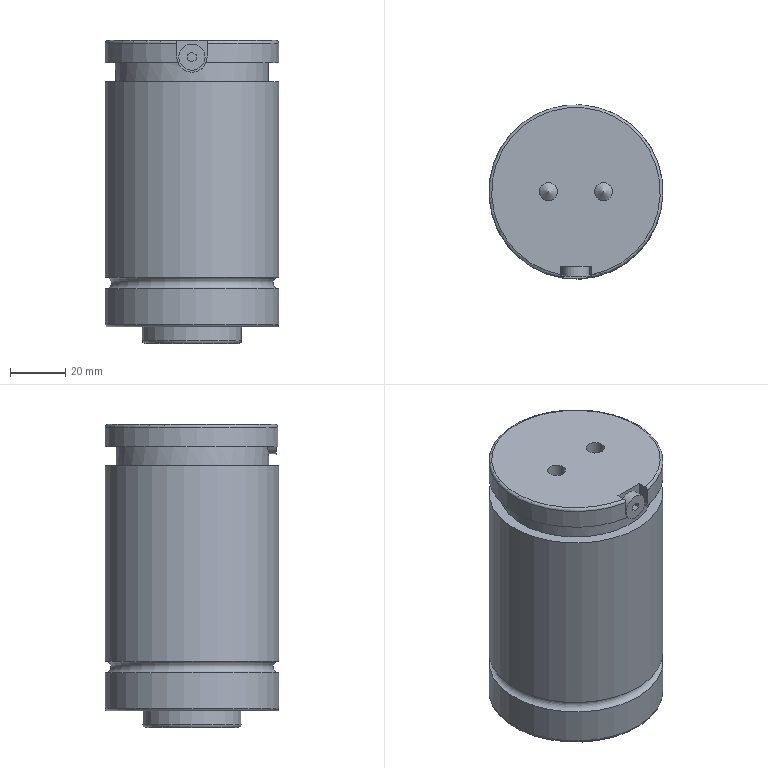Part | NX | features 1 2 | 1 solid | 34 faces | box 63.2 x 63.2 x 110 mm | volume 324925 mm3 | plane 16 | cylinder 10 | torus 4 | cone 4 | commonest cylinder face diameters 63.2 x3 6.6 x2 4.9 x1 9.5 x1 11 x1 36 x1
STEP:
#1=CARTESIAN_POINT('',(-118.4,740.,249.3));
#2=VERTEX_POINT('',#1);
#3=CARTESIAN_POINT('',(-150.,740.,249.3));
#4=DIRECTION('',(0.,0.,-1.));
#5=DIRECTION('',(1.,0.,0.));
#6=AXIS2_PLACEMENT_3D('',#3,#4,#5);
#7=CIRCLE('',#6,31.6);
#8=EDGE_CURVE('',#2,#2,#7,.T.);
#9=ORIENTED_EDGE('',*,*,#8,.T.);
#10=EDGE_LOOP('',(#9));
#11=FACE_BOUND('',#10,.T.);
#12=CARTESIAN_POINT('',(-118.4,740.,245.1));
#13=VERTEX_POINT('',#12);
#14=CARTESIAN_POINT('',(-150.,740.,245.1));
#15=DIRECTION('',(0.,0.,-1.));
#16=DIRECTION('',(1.,0.,0.));
#17=AXIS2_PLACEMENT_3D('',#14,#15,#16);
#18=CIRCLE('',#17,31.6);
#19=EDGE_CURVE('',#13,#13,#18,.T.);
#20=ORIENTED_EDGE('',*,*,#19,.F.);
#21=EDGE_LOOP('',(#20));
#22=FACE_BOUND('',#21,.T.);
#23=CARTESIAN_POINT('',(-150.,740.,247.2));
#24=DIRECTION('',(0.,0.,-1.));
#25=DIRECTION('',(0.,1.,0.));
#26=AXIS2_PLACEMENT_3D('',#23,#24,#25);
#27=TOROIDAL_SURFACE('',#26,31.6,2.1);
#28=ADVANCED_FACE('',(#11,#22),#27,.F.);
#29=CARTESIAN_POINT('',(-118.4,740.,232.2));
#30=VERTEX_POINT('',#29);
#31=CARTESIAN_POINT('',(-150.,740.,232.2));
#32=DIRECTION('',(0.,0.,-1.));
#33=DIRECTION('',(1.,0.,0.));
#34=AXIS2_PLACEMENT_3D('',#31,#32,#33);
#35=CIRCLE('',#34,31.6);
#36=EDGE_CURVE('',#30,#30,#35,.T.);
#37=ORIENTED_EDGE('',*,*,#36,.T.);
#38=EDGE_LOOP('',(#37));
#39=FACE_BOUND('',#38,.T.);
#40=CARTESIAN_POINT('',(-119.4,740.,231.2));
#41=VERTEX_POINT('',#40);
#42=CARTESIAN_POINT('',(-150.,740.,231.2));
#43=DIRECTION('',(0.,0.,-1.));
#44=DIRECTION('',(1.,0.,0.));
#45=AXIS2_PLACEMENT_3D('',#42,#43,#44);
#46=CIRCLE('',#45,30.6);
#47=EDGE_CURVE('',#41,#41,#46,.T.);
#48=ORIENTED_EDGE('',*,*,#47,.F.);
#49=EDGE_LOOP('',(#48));
#50=FACE_BOUND('',#49,.T.);
#51=CARTESIAN_POINT('',(-150.,740.,232.2));
#52=DIRECTION('',(0.,0.,-1.));
#53=DIRECTION('',(0.,1.,0.));
#54=AXIS2_PLACEMENT_3D('',#51,#52,#53);
#55=TOROIDAL_SURFACE('',#54,30.6,1.);
#56=ADVANCED_FACE('',(#39,#50),#55,.T.);
#57=ORIENTED_EDGE('',*,*,#19,.T.);
#58=EDGE_LOOP('',(#57));
#59=FACE_BOUND('',#58,.T.);
#60=ORIENTED_EDGE('',*,*,#36,.F.);
#61=EDGE_LOOP('',(#60));
#62=FACE_BOUND('',#61,.T.);
#63=CARTESIAN_POINT('',(-150.,740.,238.65));
#64=DIRECTION('',(0.,0.,1.));
#65=DIRECTION('',(0.,-1.,0.));
#66=AXIS2_PLACEMENT_3D('',#63,#64,#65);
#67=CYLINDRICAL_SURFACE('',#66,31.6);
#68=ADVANCED_FACE('',(#59,#62),#67,.T.);
#69=CARTESIAN_POINT('',(-118.4,740.,320.2));
#70=VERTEX_POINT('',#69);
#71=CARTESIAN_POINT('',(-150.,740.,320.2));
#72=DIRECTION('',(0.,0.,1.));
#73=DIRECTION('',(1.,0.,0.));
#74=AXIS2_PLACEMENT_3D('',#71,#72,#73);
#75=CIRCLE('',#74,31.6);
#76=EDGE_CURVE('',#70,#70,#75,.F.);
#77=ORIENTED_EDGE('',*,*,#76,.T.);
#78=EDGE_LOOP('',(#77));
#79=FACE_BOUND('',#78,.T.);
#80=ORIENTED_EDGE('',*,*,#8,.F.);
#81=EDGE_LOOP('',(#80));
#82=FACE_BOUND('',#81,.T.);
#83=CARTESIAN_POINT('',(-150.,740.,310.25));
#84=DIRECTION('',(0.,0.,1.));
#85=DIRECTION('',(0.,-1.,0.));
#86=AXIS2_PLACEMENT_3D('',#83,#84,#85);
#87=CYLINDRICAL_SURFACE('',#86,31.6);
#88=ADVANCED_FACE('',(#79,#82),#87,.T.);
#89=CARTESIAN_POINT('',(-122.2,740.,320.2));
#90=VERTEX_POINT('',#89);
#91=CARTESIAN_POINT('',(-150.,740.,320.2));
#92=DIRECTION('',(0.,0.,-1.));
#93=DIRECTION('',(1.,0.,0.));
#94=AXIS2_PLACEMENT_3D('',#91,#92,#93);
#95=CIRCLE('',#94,27.8);
#96=EDGE_CURVE('',#90,#90,#95,.T.);
#97=ORIENTED_EDGE('',*,*,#96,.F.);
#98=EDGE_LOOP('',(#97));
#99=FACE_BOUND('',#98,.T.);
#100=CARTESIAN_POINT('',(-155.123,712.676,327.2));
#101=VERTEX_POINT('',#100);
#102=CARTESIAN_POINT('',(-144.877,712.676,327.2));
#103=VERTEX_POINT('',#102);
#104=CARTESIAN_POINT('',(-150.,740.,327.2));
#105=DIRECTION('',(0.,0.,-1.));
#106=DIRECTION('',(1.,0.,0.));
#107=AXIS2_PLACEMENT_3D('',#104,#105,#106);
#108=CIRCLE('',#107,27.8);
#109=EDGE_CURVE('',#101,#103,#108,.T.);
#110=ORIENTED_EDGE('',*,*,#109,.T.);
#111=CARTESIAN_POINT('',(-144.877,712.676,327.2));
#112=CARTESIAN_POINT('',(-145.28,712.601,326.166));
#113=CARTESIAN_POINT('',(-146.696,712.348,324.391));
#114=CARTESIAN_POINT('',(-149.997,712.126,323.355));
#115=CARTESIAN_POINT('',(-153.301,712.348,324.388));
#116=CARTESIAN_POINT('',(-154.72,712.601,326.166));
#117=CARTESIAN_POINT('',(-155.123,712.676,327.2));
#118=B_SPLINE_CURVE_WITH_KNOTS('',3,(#111,#112,#113,#114,#115,#116,#117),.UNSPECIFIED.,.F.,.F.,(4,1,1,1,4),(0.,0.00329,0.006579,0.009869,0.01316),.UNSPECIFIED.);
#119=EDGE_CURVE('',#103,#101,#118,.T.);
#120=ORIENTED_EDGE('',*,*,#119,.T.);
#121=EDGE_LOOP('',(#110,#120));
#122=FACE_BOUND('',#121,.T.);
#123=CARTESIAN_POINT('',(-150.,740.,323.7));
#124=DIRECTION('',(0.,0.,1.));
#125=DIRECTION('',(0.,-1.,0.));
#126=AXIS2_PLACEMENT_3D('',#123,#124,#125);
#127=CYLINDRICAL_SURFACE('',#126,27.8);
#128=ADVANCED_FACE('',(#99,#122),#127,.T.);
#129=CARTESIAN_POINT('',(-132.,740.,226.2));
#130=VERTEX_POINT('',#129);
#131=CARTESIAN_POINT('',(-150.,740.,226.2));
#132=DIRECTION('',(0.,0.,-1.));
#133=DIRECTION('',(1.,0.,0.));
#134=AXIS2_PLACEMENT_3D('',#131,#132,#133);
#135=CIRCLE('',#134,18.);
#136=EDGE_CURVE('',#130,#130,#135,.T.);
#137=ORIENTED_EDGE('',*,*,#136,.T.);
#138=EDGE_LOOP('',(#137));
#139=FACE_BOUND('',#138,.T.);
#140=CARTESIAN_POINT('',(-133.,740.,225.2));
#141=VERTEX_POINT('',#140);
#142=CARTESIAN_POINT('',(-150.,740.,225.2));
#143=DIRECTION('',(0.,0.,-1.));
#144=DIRECTION('',(1.,0.,0.));
#145=AXIS2_PLACEMENT_3D('',#142,#143,#144);
#146=CIRCLE('',#145,17.);
#147=EDGE_CURVE('',#141,#141,#146,.T.);
#148=ORIENTED_EDGE('',*,*,#147,.F.);
#149=EDGE_LOOP('',(#148));
#150=FACE_BOUND('',#149,.T.);
#151=CARTESIAN_POINT('',(-150.,740.,226.2));
#152=DIRECTION('',(0.,0.,-1.));
#153=DIRECTION('',(0.,1.,0.));
#154=AXIS2_PLACEMENT_3D('',#151,#152,#153);
#155=TOROIDAL_SURFACE('',#154,17.,1.);
#156=ADVANCED_FACE('',(#139,#150),#155,.T.);
#157=CARTESIAN_POINT('',(-132.,740.,231.2));
#158=VERTEX_POINT('',#157);
#159=CARTESIAN_POINT('',(-150.,740.,231.2));
#160=DIRECTION('',(0.,0.,1.));
#161=DIRECTION('',(1.,0.,0.));
#162=AXIS2_PLACEMENT_3D('',#159,#160,#161);
#163=CIRCLE('',#162,18.);
#164=EDGE_CURVE('',#158,#158,#163,.T.);
#165=ORIENTED_EDGE('',*,*,#164,.F.);
#166=EDGE_LOOP('',(#165));
#167=FACE_BOUND('',#166,.T.);
#168=ORIENTED_EDGE('',*,*,#136,.F.);
#169=EDGE_LOOP('',(#168));
#170=FACE_BOUND('',#169,.T.);
#171=CARTESIAN_POINT('',(-150.,740.,230.2));
#172=DIRECTION('',(0.,0.,1.));
#173=DIRECTION('',(0.,-1.,0.));
#174=AXIS2_PLACEMENT_3D('',#171,#172,#173);
#175=CYLINDRICAL_SURFACE('',#174,18.);
#176=ADVANCED_FACE('',(#167,#170),#175,.T.);
#177=CARTESIAN_POINT('',(-143.3,740.,335.2));
#178=VERTEX_POINT('',#177);
#179=CARTESIAN_POINT('',(-140.,740.,335.2));
#180=DIRECTION('',(0.,0.,-1.));
#181=DIRECTION('',(-1.,0.,0.));
#182=AXIS2_PLACEMENT_3D('',#179,#180,#181);
#183=CIRCLE('',#182,3.3);
#184=EDGE_CURVE('',#178,#178,#183,.T.);
#185=ORIENTED_EDGE('',*,*,#184,.F.);
#186=EDGE_LOOP('',(#185));
#187=FACE_BOUND('',#186,.T.);
#188=CARTESIAN_POINT('',(-143.3,740.,324.));
#189=VERTEX_POINT('',#188);
#190=CARTESIAN_POINT('',(-140.,740.,324.));
#191=DIRECTION('',(0.,0.,1.));
#192=DIRECTION('',(-1.,0.,0.));
#193=AXIS2_PLACEMENT_3D('',#190,#191,#192);
#194=CIRCLE('',#193,3.3);
#195=EDGE_CURVE('',#189,#189,#194,.T.);
#196=ORIENTED_EDGE('',*,*,#195,.F.);
#197=EDGE_LOOP('',(#196));
#198=FACE_BOUND('',#197,.T.);
#199=CARTESIAN_POINT('',(-140.,740.,329.6));
#200=DIRECTION('',(0.,0.,-1.));
#201=DIRECTION('',(0.,1.,0.));
#202=AXIS2_PLACEMENT_3D('',#199,#200,#201);
#203=CYLINDRICAL_SURFACE('',#202,3.3);
#204=ADVANCED_FACE('',(#187,#198),#203,.F.);
#205=ORIENTED_EDGE('',*,*,#195,.T.);
#206=EDGE_LOOP('',(#205));
#207=FACE_BOUND('',#206,.T.);
#208=CARTESIAN_POINT('',(-140.,740.,326.7));
#209=VERTEX_POINT('',#208);
#210=VERTEX_LOOP('',#209);
#211=FACE_BOUND('',#210,.T.);
#212=CARTESIAN_POINT('',(-140.,740.,325.35));
#213=DIRECTION('',(0.,0.,-1.));
#214=DIRECTION('',(0.,1.,0.));
#215=AXIS2_PLACEMENT_3D('',#212,#213,#214);
#216=CONICAL_SURFACE('',#215,1.65,0.8851);
#217=ADVANCED_FACE('',(#207,#211),#216,.T.);
#218=CARTESIAN_POINT('',(-146.5,740.,225.2));
#219=VERTEX_POINT('',#218);
#220=CARTESIAN_POINT('',(-150.,740.,225.2));
#221=DIRECTION('',(0.,0.,1.));
#222=DIRECTION('',(1.,0.,0.));
#223=AXIS2_PLACEMENT_3D('',#220,#221,#222);
#224=CIRCLE('',#223,3.5);
#225=EDGE_CURVE('',#219,#219,#224,.T.);
#226=ORIENTED_EDGE('',*,*,#225,.F.);
#227=EDGE_LOOP('',(#226));
#228=FACE_BOUND('',#227,.T.);
#229=CARTESIAN_POINT('',(-147.55,740.,226.25));
#230=VERTEX_POINT('',#229);
#231=CARTESIAN_POINT('',(-150.,740.,226.25));
#232=DIRECTION('',(0.,0.,-1.));
#233=DIRECTION('',(1.,0.,0.));
#234=AXIS2_PLACEMENT_3D('',#231,#232,#233);
#235=CIRCLE('',#234,2.45);
#236=EDGE_CURVE('',#230,#230,#235,.T.);
#237=ORIENTED_EDGE('',*,*,#236,.F.);
#238=EDGE_LOOP('',(#237));
#239=FACE_BOUND('',#238,.T.);
#240=CARTESIAN_POINT('',(-150.,740.,225.725));
#241=DIRECTION('',(0.,0.,-1.));
#242=DIRECTION('',(0.,1.,0.));
#243=AXIS2_PLACEMENT_3D('',#240,#241,#242);
#244=CONICAL_SURFACE('',#243,2.975,0.7854);
#245=ADVANCED_FACE('',(#228,#239),#244,.F.);
#246=ORIENTED_EDGE('',*,*,#236,.T.);
#247=EDGE_LOOP('',(#246));
#248=FACE_BOUND('',#247,.T.);
#249=CARTESIAN_POINT('',(-147.55,740.,231.7));
#250=VERTEX_POINT('',#249);
#251=CARTESIAN_POINT('',(-150.,740.,231.7));
#252=DIRECTION('',(0.,0.,-1.));
#253=DIRECTION('',(1.,0.,0.));
#254=AXIS2_PLACEMENT_3D('',#251,#252,#253);
#255=CIRCLE('',#254,2.45);
#256=EDGE_CURVE('',#250,#250,#255,.T.);
#257=ORIENTED_EDGE('',*,*,#256,.F.);
#258=EDGE_LOOP('',(#257));
#259=FACE_BOUND('',#258,.T.);
#260=CARTESIAN_POINT('',(-150.,740.,228.975));
#261=DIRECTION('',(0.,0.,1.));
#262=DIRECTION('',(0.,-1.,0.));
#263=AXIS2_PLACEMENT_3D('',#260,#261,#262);
#264=CYLINDRICAL_SURFACE('',#263,2.45);
#265=ADVANCED_FACE('',(#248,#259),#264,.F.);
#266=CARTESIAN_POINT('',(-150.,740.,232.7));
#267=VERTEX_POINT('',#266);
#268=VERTEX_LOOP('',#267);
#269=FACE_BOUND('',#268,.T.);
#270=ORIENTED_EDGE('',*,*,#256,.T.);
#271=EDGE_LOOP('',(#270));
#272=FACE_BOUND('',#271,.T.);
#273=CARTESIAN_POINT('',(-150.,740.,232.2));
#274=DIRECTION('',(0.,0.,-1.));
#275=DIRECTION('',(0.,1.,0.));
#276=AXIS2_PLACEMENT_3D('',#273,#274,#275);
#277=CONICAL_SURFACE('',#276,1.225,1.183);
#278=ADVANCED_FACE('',(#269,#272),#277,.F.);
#279=CARTESIAN_POINT('',(-160.,740.,326.7));
#280=VERTEX_POINT('',#279);
#281=VERTEX_LOOP('',#280);
#282=FACE_BOUND('',#281,.T.);
#283=CARTESIAN_POINT('',(-156.7,740.,324.));
#284=VERTEX_POINT('',#283);
#285=CARTESIAN_POINT('',(-160.,740.,324.));
#286=DIRECTION('',(0.,0.,-1.));
#287=DIRECTION('',(1.,0.,0.));
#288=AXIS2_PLACEMENT_3D('',#285,#286,#287);
#289=CIRCLE('',#288,3.3);
#290=EDGE_CURVE('',#284,#284,#289,.T.);
#291=ORIENTED_EDGE('',*,*,#290,.F.);
#292=EDGE_LOOP('',(#291));
#293=FACE_BOUND('',#292,.T.);
#294=CARTESIAN_POINT('',(-160.,740.,325.35));
#295=DIRECTION('',(0.,0.,-1.));
#296=DIRECTION('',(0.,1.,0.));
#297=AXIS2_PLACEMENT_3D('',#294,#295,#296);
#298=CONICAL_SURFACE('',#297,1.65,0.8851);
#299=ADVANCED_FACE('',(#282,#293),#298,.T.);
#300=ORIENTED_EDGE('',*,*,#290,.T.);
#301=EDGE_LOOP('',(#300));
#302=FACE_BOUND('',#301,.T.);
#303=CARTESIAN_POINT('',(-156.7,740.,335.2));
#304=VERTEX_POINT('',#303);
#305=CARTESIAN_POINT('',(-160.,740.,335.2));
#306=DIRECTION('',(0.,0.,-1.));
#307=DIRECTION('',(1.,0.,0.));
#308=AXIS2_PLACEMENT_3D('',#305,#306,#307);
#309=CIRCLE('',#308,3.3);
#310=EDGE_CURVE('',#304,#304,#309,.T.);
#311=ORIENTED_EDGE('',*,*,#310,.F.);
#312=EDGE_LOOP('',(#311));
#313=FACE_BOUND('',#312,.T.);
#314=CARTESIAN_POINT('',(-160.,740.,329.6));
#315=DIRECTION('',(0.,0.,1.));
#316=DIRECTION('',(0.,-1.,0.));
#317=AXIS2_PLACEMENT_3D('',#314,#315,#316);
#318=CYLINDRICAL_SURFACE('',#317,3.3);
#319=ADVANCED_FACE('',(#302,#313),#318,.F.);
#320=CARTESIAN_POINT('',(-155.5,708.882,334.2));
#321=VERTEX_POINT('',#320);
#322=CARTESIAN_POINT('',(-144.5,708.882,334.2));
#323=VERTEX_POINT('',#322);
#324=CARTESIAN_POINT('',(-150.,740.,334.2));
#325=DIRECTION('',(0.,0.,-1.));
#326=DIRECTION('',(1.,0.,0.));
#327=AXIS2_PLACEMENT_3D('',#324,#325,#326);
#328=CIRCLE('',#327,31.6);
#329=EDGE_CURVE('',#321,#323,#328,.T.);
#330=ORIENTED_EDGE('',*,*,#329,.T.);
#331=CARTESIAN_POINT('',(-144.5,708.882,329.2));
#332=VERTEX_POINT('',#331);
#333=CARTESIAN_POINT('',(-144.5,708.882,331.7));
#334=DIRECTION('',(0.,0.,-1.));
#335=VECTOR('',#334,1000.);
#336=LINE('',#333,#335);
#337=EDGE_CURVE('',#323,#332,#336,.T.);
#338=ORIENTED_EDGE('',*,*,#337,.T.);
#339=CARTESIAN_POINT('',(-144.877,708.818,327.2));
#340=VERTEX_POINT('',#339);
#341=CARTESIAN_POINT('',(-144.5,708.882,329.2));
#342=CARTESIAN_POINT('',(-144.5,708.882,328.509));
#343=CARTESIAN_POINT('',(-144.626,708.859,327.842));
#344=CARTESIAN_POINT('',(-144.877,708.818,327.2));
#345=B_SPLINE_CURVE_WITH_KNOTS('',3,(#341,#342,#343,#344),.UNSPECIFIED.,.F.,.F.,(4,4),(0.,0.002036),.UNSPECIFIED.);
#346=EDGE_CURVE('',#332,#340,#345,.T.);
#347=ORIENTED_EDGE('',*,*,#346,.T.);
#348=CARTESIAN_POINT('',(-155.123,708.818,327.2));
#349=VERTEX_POINT('',#348);
#350=CARTESIAN_POINT('',(-150.,740.,327.2));
#351=DIRECTION('',(0.,0.,1.));
#352=DIRECTION('',(1.,0.,0.));
#353=AXIS2_PLACEMENT_3D('',#350,#351,#352);
#354=CIRCLE('',#353,31.6);
#355=EDGE_CURVE('',#340,#349,#354,.T.);
#356=ORIENTED_EDGE('',*,*,#355,.T.);
#357=CARTESIAN_POINT('',(-155.5,708.882,329.2));
#358=VERTEX_POINT('',#357);
#359=CARTESIAN_POINT('',(-155.123,708.818,327.2));
#360=CARTESIAN_POINT('',(-155.374,708.859,327.842));
#361=CARTESIAN_POINT('',(-155.5,708.882,328.509));
#362=CARTESIAN_POINT('',(-155.5,708.882,329.2));
#363=B_SPLINE_CURVE_WITH_KNOTS('',3,(#359,#360,#361,#362),.UNSPECIFIED.,.F.,.F.,(4,4),(0.,0.002036),.UNSPECIFIED.);
#364=EDGE_CURVE('',#349,#358,#363,.T.);
#365=ORIENTED_EDGE('',*,*,#364,.T.);
#366=CARTESIAN_POINT('',(-155.5,708.882,331.7));
#367=DIRECTION('',(0.,0.,1.));
#368=VECTOR('',#367,1000.);
#369=LINE('',#366,#368);
#370=EDGE_CURVE('',#358,#321,#369,.T.);
#371=ORIENTED_EDGE('',*,*,#370,.T.);
#372=EDGE_LOOP('',(#330,#338,#347,#356,#365,#371));
#373=FACE_BOUND('',#372,.T.);
#374=CARTESIAN_POINT('',(-150.,740.,273.25));
#375=DIRECTION('',(0.,0.,1.));
#376=DIRECTION('',(0.,-1.,0.));
#377=AXIS2_PLACEMENT_3D('',#374,#375,#376);
#378=CYLINDRICAL_SURFACE('',#377,31.6);
#379=ADVANCED_FACE('',(#373),#378,.T.);
#380=CARTESIAN_POINT('',(-144.5,709.898,335.2));
#381=VERTEX_POINT('',#380);
#382=CARTESIAN_POINT('',(-144.5,709.898,335.2));
#383=CARTESIAN_POINT('',(-144.5,709.366,335.2));
#384=CARTESIAN_POINT('',(-144.5,708.882,334.733));
#385=CARTESIAN_POINT('',(-144.5,708.882,334.2));
#386=B_SPLINE_CURVE_WITH_KNOTS('',3,(#382,#383,#384,#385),.UNSPECIFIED.,.F.,.F.,(4,4),(0.,0.001575),.UNSPECIFIED.);
#387=EDGE_CURVE('',#381,#323,#386,.T.);
#388=ORIENTED_EDGE('',*,*,#387,.T.);
#389=ORIENTED_EDGE('',*,*,#329,.F.);
#390=CARTESIAN_POINT('',(-155.5,709.898,335.2));
#391=VERTEX_POINT('',#390);
#392=CARTESIAN_POINT('',(-155.5,708.882,334.2));
#393=CARTESIAN_POINT('',(-155.5,708.882,334.733));
#394=CARTESIAN_POINT('',(-155.5,709.366,335.2));
#395=CARTESIAN_POINT('',(-155.5,709.898,335.2));
#396=B_SPLINE_CURVE_WITH_KNOTS('',3,(#392,#393,#394,#395),.UNSPECIFIED.,.F.,.F.,(4,4),(0.,0.001575),.UNSPECIFIED.);
#397=EDGE_CURVE('',#321,#391,#396,.T.);
#398=ORIENTED_EDGE('',*,*,#397,.T.);
#399=CARTESIAN_POINT('',(-150.,740.,335.2));
#400=DIRECTION('',(0.,0.,-1.));
#401=DIRECTION('',(1.,0.,0.));
#402=AXIS2_PLACEMENT_3D('',#399,#400,#401);
#403=CIRCLE('',#402,30.6);
#404=EDGE_CURVE('',#391,#381,#403,.T.);
#405=ORIENTED_EDGE('',*,*,#404,.T.);
#406=EDGE_LOOP('',(#388,#389,#398,#405));
#407=FACE_BOUND('',#406,.T.);
#408=CARTESIAN_POINT('',(-150.,740.,334.2));
#409=DIRECTION('',(0.,0.,-1.));
#410=DIRECTION('',(0.,1.,0.));
#411=AXIS2_PLACEMENT_3D('',#408,#409,#410);
#412=TOROIDAL_SURFACE('',#411,30.6,1.);
#413=ADVANCED_FACE('',(#407),#412,.T.);
#414=CARTESIAN_POINT('',(-145.25,712.9,329.2));
#415=VERTEX_POINT('',#414);
#416=CARTESIAN_POINT('',(-150.,712.9,329.2));
#417=DIRECTION('',(0.,1.,0.));
#418=DIRECTION('',(1.,0.,0.));
#419=AXIS2_PLACEMENT_3D('',#416,#417,#418);
#420=CIRCLE('',#419,4.75);
#421=EDGE_CURVE('',#415,#415,#420,.T.);
#422=ORIENTED_EDGE('',*,*,#421,.F.);
#423=EDGE_LOOP('',(#422));
#424=FACE_BOUND('',#423,.T.);
#425=CARTESIAN_POINT('',(-145.25,709.4,329.2));
#426=VERTEX_POINT('',#425);
#427=CARTESIAN_POINT('',(-150.,709.4,329.2));
#428=DIRECTION('',(0.,1.,0.));
#429=DIRECTION('',(1.,0.,0.));
#430=AXIS2_PLACEMENT_3D('',#427,#428,#429);
#431=CIRCLE('',#430,4.75);
#432=EDGE_CURVE('',#426,#426,#431,.T.);
#433=ORIENTED_EDGE('',*,*,#432,.T.);
#434=EDGE_LOOP('',(#433));
#435=FACE_BOUND('',#434,.T.);
#436=CARTESIAN_POINT('',(-150.,740.,329.2));
#437=DIRECTION('',(0.,1.,0.));
#438=DIRECTION('',(1.,0.,0.));
#439=AXIS2_PLACEMENT_3D('',#436,#437,#438);
#440=CYLINDRICAL_SURFACE('',#439,4.75);
#441=ADVANCED_FACE('',(#424,#435),#440,.T.);
#442=CARTESIAN_POINT('',(-148.5,714.4,330.066));
#443=VERTEX_POINT('',#442);
#444=CARTESIAN_POINT('',(-150.,714.4,330.932));
#445=VERTEX_POINT('',#444);
#446=CARTESIAN_POINT('',(-148.5,714.4,330.066));
#447=DIRECTION('',(-0.866,0.,0.5));
#448=VECTOR('',#447,1000.);
#449=LINE('',#446,#448);
#450=EDGE_CURVE('',#443,#445,#449,.T.);
#451=ORIENTED_EDGE('',*,*,#450,.F.);
#452=CARTESIAN_POINT('',(-148.5,709.4,330.066));
#453=VERTEX_POINT('',#452);
#454=CARTESIAN_POINT('',(-148.5,709.4,330.066));
#455=DIRECTION('',(0.,1.,0.));
#456=VECTOR('',#455,1000.);
#457=LINE('',#454,#456);
#458=EDGE_CURVE('',#453,#443,#457,.T.);
#459=ORIENTED_EDGE('',*,*,#458,.F.);
#460=CARTESIAN_POINT('',(-150.,709.4,330.932));
#461=VERTEX_POINT('',#460);
#462=CARTESIAN_POINT('',(-150.174,709.4,331.033));
#463=DIRECTION('',(0.866,0.,-0.5));
#464=VECTOR('',#463,1000.);
#465=LINE('',#462,#464);
#466=EDGE_CURVE('',#461,#453,#465,.T.);
#467=ORIENTED_EDGE('',*,*,#466,.F.);
#468=CARTESIAN_POINT('',(-150.,709.4,330.932));
#469=DIRECTION('',(0.,1.,0.));
#470=VECTOR('',#469,1000.);
#471=LINE('',#468,#470);
#472=EDGE_CURVE('',#461,#445,#471,.T.);
#473=ORIENTED_EDGE('',*,*,#472,.T.);
#474=EDGE_LOOP('',(#451,#459,#467,#473));
#475=FACE_BOUND('',#474,.T.);
#476=CARTESIAN_POINT('',(-148.5,709.4,330.066));
#477=DIRECTION('',(0.5,0.,0.866));
#478=DIRECTION('',(0.866,0.,-0.5));
#479=AXIS2_PLACEMENT_3D('',#476,#477,#478);
#480=PLANE('',#479);
#481=ADVANCED_FACE('',(#475),#480,.F.);
#482=CARTESIAN_POINT('',(-151.5,714.4,330.066));
#483=VERTEX_POINT('',#482);
#484=CARTESIAN_POINT('',(-150.,714.4,330.932));
#485=DIRECTION('',(-0.866,0.,-0.5));
#486=VECTOR('',#485,1000.);
#487=LINE('',#484,#486);
#488=EDGE_CURVE('',#445,#483,#487,.T.);
#489=ORIENTED_EDGE('',*,*,#488,.F.);
#490=ORIENTED_EDGE('',*,*,#472,.F.);
#491=CARTESIAN_POINT('',(-151.5,709.4,330.066));
#492=VERTEX_POINT('',#491);
#493=CARTESIAN_POINT('',(-149.076,709.4,331.466));
#494=DIRECTION('',(0.866,0.,0.5));
#495=VECTOR('',#494,1000.);
#496=LINE('',#493,#495);
#497=EDGE_CURVE('',#492,#461,#496,.T.);
#498=ORIENTED_EDGE('',*,*,#497,.F.);
#499=CARTESIAN_POINT('',(-151.5,709.4,330.066));
#500=DIRECTION('',(0.,1.,0.));
#501=VECTOR('',#500,1000.);
#502=LINE('',#499,#501);
#503=EDGE_CURVE('',#492,#483,#502,.T.);
#504=ORIENTED_EDGE('',*,*,#503,.T.);
#505=EDGE_LOOP('',(#489,#490,#498,#504));
#506=FACE_BOUND('',#505,.T.);
#507=CARTESIAN_POINT('',(-150.,709.4,330.932));
#508=DIRECTION('',(-0.5,0.,0.866));
#509=DIRECTION('',(0.866,0.,0.5));
#510=AXIS2_PLACEMENT_3D('',#507,#508,#509);
#511=PLANE('',#510);
#512=ADVANCED_FACE('',(#506),#511,.F.);
#513=CARTESIAN_POINT('',(-151.5,714.4,328.334));
#514=VERTEX_POINT('',#513);
#515=CARTESIAN_POINT('',(-151.5,714.4,330.066));
#516=DIRECTION('',(0.,0.,-1.));
#517=VECTOR('',#516,1000.);
#518=LINE('',#515,#517);
#519=EDGE_CURVE('',#483,#514,#518,.T.);
#520=ORIENTED_EDGE('',*,*,#519,.F.);
#521=ORIENTED_EDGE('',*,*,#503,.F.);
#522=CARTESIAN_POINT('',(-151.5,709.4,328.334));
#523=VERTEX_POINT('',#522);
#524=CARTESIAN_POINT('',(-151.5,709.4,332.633));
#525=DIRECTION('',(0.,0.,1.));
#526=VECTOR('',#525,1000.);
#527=LINE('',#524,#526);
#528=EDGE_CURVE('',#523,#492,#527,.T.);
#529=ORIENTED_EDGE('',*,*,#528,.F.);
#530=CARTESIAN_POINT('',(-151.5,709.4,328.334));
#531=DIRECTION('',(0.,1.,0.));
#532=VECTOR('',#531,1000.);
#533=LINE('',#530,#532);
#534=EDGE_CURVE('',#523,#514,#533,.T.);
#535=ORIENTED_EDGE('',*,*,#534,.T.);
#536=EDGE_LOOP('',(#520,#521,#529,#535));
#537=FACE_BOUND('',#536,.T.);
#538=CARTESIAN_POINT('',(-151.5,709.4,330.066));
#539=DIRECTION('',(-1.,0.,0.));
#540=DIRECTION('',(0.,1.,0.));
#541=AXIS2_PLACEMENT_3D('',#538,#539,#540);
#542=PLANE('',#541);
#543=ADVANCED_FACE('',(#537),#542,.F.);
#544=CARTESIAN_POINT('',(-150.,714.4,327.468));
#545=VERTEX_POINT('',#544);
#546=CARTESIAN_POINT('',(-151.5,714.4,328.334));
#547=DIRECTION('',(0.866,0.,-0.5));
#548=VECTOR('',#547,1000.);
#549=LINE('',#546,#548);
#550=EDGE_CURVE('',#514,#545,#549,.T.);
#551=ORIENTED_EDGE('',*,*,#550,.F.);
#552=ORIENTED_EDGE('',*,*,#534,.F.);
#553=CARTESIAN_POINT('',(-150.,709.4,327.468));
#554=VERTEX_POINT('',#553);
#555=CARTESIAN_POINT('',(-152.424,709.4,328.867));
#556=DIRECTION('',(-0.866,0.,0.5));
#557=VECTOR('',#556,1000.);
#558=LINE('',#555,#557);
#559=EDGE_CURVE('',#554,#523,#558,.T.);
#560=ORIENTED_EDGE('',*,*,#559,.F.);
#561=CARTESIAN_POINT('',(-150.,709.4,327.468));
#562=DIRECTION('',(0.,1.,0.));
#563=VECTOR('',#562,1000.);
#564=LINE('',#561,#563);
#565=EDGE_CURVE('',#554,#545,#564,.T.);
#566=ORIENTED_EDGE('',*,*,#565,.T.);
#567=EDGE_LOOP('',(#551,#552,#560,#566));
#568=FACE_BOUND('',#567,.T.);
#569=CARTESIAN_POINT('',(-151.5,709.4,328.334));
#570=DIRECTION('',(-0.5,0.,-0.866));
#571=DIRECTION('',(-0.866,0.,0.5));
#572=AXIS2_PLACEMENT_3D('',#569,#570,#571);
#573=PLANE('',#572);
#574=ADVANCED_FACE('',(#568),#573,.F.);
#575=CARTESIAN_POINT('',(-148.5,714.4,328.334));
#576=VERTEX_POINT('',#575);
#577=CARTESIAN_POINT('',(-150.,714.4,327.468));
#578=DIRECTION('',(0.866,0.,0.5));
#579=VECTOR('',#578,1000.);
#580=LINE('',#577,#579);
#581=EDGE_CURVE('',#545,#576,#580,.T.);
#582=ORIENTED_EDGE('',*,*,#581,.F.);
#583=ORIENTED_EDGE('',*,*,#565,.F.);
#584=CARTESIAN_POINT('',(-148.5,709.4,328.334));
#585=VERTEX_POINT('',#584);
#586=CARTESIAN_POINT('',(-148.326,709.4,328.434));
#587=DIRECTION('',(-0.866,0.,-0.5));
#588=VECTOR('',#587,1000.);
#589=LINE('',#586,#588);
#590=EDGE_CURVE('',#585,#554,#589,.T.);
#591=ORIENTED_EDGE('',*,*,#590,.F.);
#592=CARTESIAN_POINT('',(-148.5,709.4,328.334));
#593=DIRECTION('',(0.,1.,0.));
#594=VECTOR('',#593,1000.);
#595=LINE('',#592,#594);
#596=EDGE_CURVE('',#585,#576,#595,.T.);
#597=ORIENTED_EDGE('',*,*,#596,.T.);
#598=EDGE_LOOP('',(#582,#583,#591,#597));
#599=FACE_BOUND('',#598,.T.);
#600=CARTESIAN_POINT('',(-150.,709.4,327.468));
#601=DIRECTION('',(0.5,0.,-0.866));
#602=DIRECTION('',(-0.866,0.,-0.5));
#603=AXIS2_PLACEMENT_3D('',#600,#601,#602);
#604=PLANE('',#603);
#605=ADVANCED_FACE('',(#599),#604,.F.);
#606=CARTESIAN_POINT('',(-148.5,714.4,328.334));
#607=DIRECTION('',(0.,0.,1.));
#608=VECTOR('',#607,1000.);
#609=LINE('',#606,#608);
#610=EDGE_CURVE('',#576,#443,#609,.T.);
#611=ORIENTED_EDGE('',*,*,#610,.F.);
#612=ORIENTED_EDGE('',*,*,#596,.F.);
#613=CARTESIAN_POINT('',(-148.5,709.4,331.767));
#614=DIRECTION('',(0.,0.,-1.));
#615=VECTOR('',#614,1000.);
#616=LINE('',#613,#615);
#617=EDGE_CURVE('',#453,#585,#616,.T.);
#618=ORIENTED_EDGE('',*,*,#617,.F.);
#619=ORIENTED_EDGE('',*,*,#458,.T.);
#620=EDGE_LOOP('',(#611,#612,#618,#619));
#621=FACE_BOUND('',#620,.T.);
#622=CARTESIAN_POINT('',(-148.5,709.4,328.334));
#623=DIRECTION('',(1.,0.,0.));
#624=DIRECTION('',(0.,-1.,0.));
#625=AXIS2_PLACEMENT_3D('',#622,#623,#624);
#626=PLANE('',#625);
#627=ADVANCED_FACE('',(#621),#626,.F.);
#628=ORIENTED_EDGE('',*,*,#450,.T.);
#629=ORIENTED_EDGE('',*,*,#488,.T.);
#630=ORIENTED_EDGE('',*,*,#519,.T.);
#631=ORIENTED_EDGE('',*,*,#550,.T.);
#632=ORIENTED_EDGE('',*,*,#581,.T.);
#633=ORIENTED_EDGE('',*,*,#610,.T.);
#634=EDGE_LOOP('',(#628,#629,#630,#631,#632,#633));
#635=FACE_BOUND('',#634,.T.);
#636=CARTESIAN_POINT('',(-150.,714.4,329.2));
#637=DIRECTION('',(0.,-1.,0.));
#638=DIRECTION('',(-1.,0.,0.));
#639=AXIS2_PLACEMENT_3D('',#636,#637,#638);
#640=PLANE('',#639);
#641=ADVANCED_FACE('',(#635),#640,.T.);
#642=ORIENTED_EDGE('',*,*,#466,.T.);
#643=ORIENTED_EDGE('',*,*,#617,.T.);
#644=ORIENTED_EDGE('',*,*,#590,.T.);
#645=ORIENTED_EDGE('',*,*,#559,.T.);
#646=ORIENTED_EDGE('',*,*,#528,.T.);
#647=ORIENTED_EDGE('',*,*,#497,.T.);
#648=EDGE_LOOP('',(#642,#643,#644,#645,#646,#647));
#649=FACE_BOUND('',#648,.T.);
#650=ORIENTED_EDGE('',*,*,#432,.F.);
#651=EDGE_LOOP('',(#650));
#652=FACE_BOUND('',#651,.T.);
#653=CARTESIAN_POINT('',(-150.,709.4,335.2));
#654=DIRECTION('',(0.,1.,0.));
#655=DIRECTION('',(1.,0.,0.));
#656=AXIS2_PLACEMENT_3D('',#653,#654,#655);
#657=PLANE('',#656);
#658=ADVANCED_FACE('',(#649,#652),#657,.F.);
#659=ORIENTED_EDGE('',*,*,#370,.F.);
#660=CARTESIAN_POINT('',(-155.5,712.9,329.2));
#661=VERTEX_POINT('',#660);
#662=CARTESIAN_POINT('',(-155.5,708.4,329.2));
#663=DIRECTION('',(0.,1.,0.));
#664=VECTOR('',#663,1000.);
#665=LINE('',#662,#664);
#666=EDGE_CURVE('',#358,#661,#665,.T.);
#667=ORIENTED_EDGE('',*,*,#666,.T.);
#668=CARTESIAN_POINT('',(-155.5,712.9,335.2));
#669=VERTEX_POINT('',#668);
#670=CARTESIAN_POINT('',(-155.5,712.9,329.2));
#671=DIRECTION('',(0.,0.,-1.));
#672=VECTOR('',#671,1000.);
#673=LINE('',#670,#672);
#674=EDGE_CURVE('',#669,#661,#673,.T.);
#675=ORIENTED_EDGE('',*,*,#674,.F.);
#676=CARTESIAN_POINT('',(-155.5,724.2,335.2));
#677=DIRECTION('',(0.,1.,0.));
#678=VECTOR('',#677,1000.);
#679=LINE('',#676,#678);
#680=EDGE_CURVE('',#391,#669,#679,.T.);
#681=ORIENTED_EDGE('',*,*,#680,.F.);
#682=ORIENTED_EDGE('',*,*,#397,.F.);
#683=EDGE_LOOP('',(#659,#667,#675,#681,#682));
#684=FACE_BOUND('',#683,.T.);
#685=CARTESIAN_POINT('',(-155.5,708.4,335.2));
#686=DIRECTION('',(-1.,0.,0.));
#687=DIRECTION('',(0.,1.,0.));
#688=AXIS2_PLACEMENT_3D('',#685,#686,#687);
#689=PLANE('',#688);
#690=ADVANCED_FACE('',(#684),#689,.F.);
#691=ORIENTED_EDGE('',*,*,#364,.F.);
#692=CARTESIAN_POINT('',(-155.123,710.65,327.2));
#693=DIRECTION('',(0.,-1.,0.));
#694=VECTOR('',#693,1000.);
#695=LINE('',#692,#694);
#696=EDGE_CURVE('',#101,#349,#695,.T.);
#697=ORIENTED_EDGE('',*,*,#696,.F.);
#698=ORIENTED_EDGE('',*,*,#119,.F.);
#699=CARTESIAN_POINT('',(-144.877,710.65,327.2));
#700=DIRECTION('',(0.,1.,0.));
#701=VECTOR('',#700,1000.);
#702=LINE('',#699,#701);
#703=EDGE_CURVE('',#340,#103,#702,.T.);
#704=ORIENTED_EDGE('',*,*,#703,.F.);
#705=ORIENTED_EDGE('',*,*,#346,.F.);
#706=CARTESIAN_POINT('',(-144.5,712.9,329.2));
#707=VERTEX_POINT('',#706);
#708=CARTESIAN_POINT('',(-144.5,708.4,329.2));
#709=DIRECTION('',(0.,1.,0.));
#710=VECTOR('',#709,1000.);
#711=LINE('',#708,#710);
#712=EDGE_CURVE('',#332,#707,#711,.T.);
#713=ORIENTED_EDGE('',*,*,#712,.T.);
#714=CARTESIAN_POINT('',(-150.,712.9,329.2));
#715=DIRECTION('',(0.,-1.,0.));
#716=DIRECTION('',(1.,0.,0.));
#717=AXIS2_PLACEMENT_3D('',#714,#715,#716);
#718=CIRCLE('',#717,5.5);
#719=EDGE_CURVE('',#661,#707,#718,.T.);
#720=ORIENTED_EDGE('',*,*,#719,.F.);
#721=ORIENTED_EDGE('',*,*,#666,.F.);
#722=EDGE_LOOP('',(#691,#697,#698,#704,#705,#713,#720,#721));
#723=FACE_BOUND('',#722,.T.);
#724=CARTESIAN_POINT('',(-150.,708.4,329.2));
#725=DIRECTION('',(0.,-1.,0.));
#726=DIRECTION('',(-1.,0.,0.));
#727=AXIS2_PLACEMENT_3D('',#724,#725,#726);
#728=CYLINDRICAL_SURFACE('',#727,5.5);
#729=ADVANCED_FACE('',(#723),#728,.F.);
#730=ORIENTED_EDGE('',*,*,#337,.F.);
#731=ORIENTED_EDGE('',*,*,#387,.F.);
#732=CARTESIAN_POINT('',(-144.5,712.9,335.2));
#733=VERTEX_POINT('',#732);
#734=CARTESIAN_POINT('',(-144.5,724.2,335.2));
#735=DIRECTION('',(0.,-1.,0.));
#736=VECTOR('',#735,1000.);
#737=LINE('',#734,#736);
#738=EDGE_CURVE('',#733,#381,#737,.T.);
#739=ORIENTED_EDGE('',*,*,#738,.F.);
#740=CARTESIAN_POINT('',(-144.5,712.9,335.2));
#741=DIRECTION('',(0.,0.,1.));
#742=VECTOR('',#741,1000.);
#743=LINE('',#740,#742);
#744=EDGE_CURVE('',#707,#733,#743,.T.);
#745=ORIENTED_EDGE('',*,*,#744,.F.);
#746=ORIENTED_EDGE('',*,*,#712,.F.);
#747=EDGE_LOOP('',(#730,#731,#739,#745,#746));
#748=FACE_BOUND('',#747,.T.);
#749=CARTESIAN_POINT('',(-144.5,708.4,329.2));
#750=DIRECTION('',(1.,0.,0.));
#751=DIRECTION('',(0.,-1.,0.));
#752=AXIS2_PLACEMENT_3D('',#749,#750,#751);
#753=PLANE('',#752);
#754=ADVANCED_FACE('',(#748),#753,.F.);
#755=ORIENTED_EDGE('',*,*,#421,.T.);
#756=EDGE_LOOP('',(#755));
#757=FACE_BOUND('',#756,.T.);
#758=ORIENTED_EDGE('',*,*,#674,.T.);
#759=ORIENTED_EDGE('',*,*,#719,.T.);
#760=ORIENTED_EDGE('',*,*,#744,.T.);
#761=CARTESIAN_POINT('',(-142.35,712.9,335.2));
#762=DIRECTION('',(1.,0.,0.));
#763=VECTOR('',#762,1000.);
#764=LINE('',#761,#763);
#765=EDGE_CURVE('',#669,#733,#764,.T.);
#766=ORIENTED_EDGE('',*,*,#765,.F.);
#767=EDGE_LOOP('',(#758,#759,#760,#766));
#768=FACE_BOUND('',#767,.T.);
#769=CARTESIAN_POINT('',(-150.,712.9,335.2));
#770=DIRECTION('',(0.,1.,0.));
#771=DIRECTION('',(1.,0.,0.));
#772=AXIS2_PLACEMENT_3D('',#769,#770,#771);
#773=PLANE('',#772);
#774=ADVANCED_FACE('',(#757,#768),#773,.F.);
#775=ORIENTED_EDGE('',*,*,#696,.T.);
#776=ORIENTED_EDGE('',*,*,#355,.F.);
#777=ORIENTED_EDGE('',*,*,#703,.T.);
#778=ORIENTED_EDGE('',*,*,#109,.F.);
#779=EDGE_LOOP('',(#775,#776,#777,#778));
#780=FACE_BOUND('',#779,.T.);
#781=CARTESIAN_POINT('',(-120.2,740.,327.2));
#782=DIRECTION('',(0.,0.,1.));
#783=DIRECTION('',(0.,-1.,0.));
#784=AXIS2_PLACEMENT_3D('',#781,#782,#783);
#785=PLANE('',#784);
#786=ADVANCED_FACE('',(#780),#785,.F.);
#787=ORIENTED_EDGE('',*,*,#680,.T.);
#788=ORIENTED_EDGE('',*,*,#765,.T.);
#789=ORIENTED_EDGE('',*,*,#738,.T.);
#790=ORIENTED_EDGE('',*,*,#404,.F.);
#791=EDGE_LOOP('',(#787,#788,#789,#790));
#792=FACE_BOUND('',#791,.T.);
#793=ORIENTED_EDGE('',*,*,#184,.T.);
#794=EDGE_LOOP('',(#793));
#795=FACE_BOUND('',#794,.T.);
#796=ORIENTED_EDGE('',*,*,#310,.T.);
#797=EDGE_LOOP('',(#796));
#798=FACE_BOUND('',#797,.T.);
#799=CARTESIAN_POINT('',(-134.7,740.,335.2));
#800=DIRECTION('',(0.,0.,1.));
#801=DIRECTION('',(1.,0.,0.));
#802=AXIS2_PLACEMENT_3D('',#799,#800,#801);
#803=PLANE('',#802);
#804=ADVANCED_FACE('',(#792,#795,#798),#803,.T.);
#805=ORIENTED_EDGE('',*,*,#225,.T.);
#806=EDGE_LOOP('',(#805));
#807=FACE_BOUND('',#806,.T.);
#808=ORIENTED_EDGE('',*,*,#147,.T.);
#809=EDGE_LOOP('',(#808));
#810=FACE_BOUND('',#809,.T.);
#811=CARTESIAN_POINT('',(-141.5,740.,225.2));
#812=DIRECTION('',(0.,0.,-1.));
#813=DIRECTION('',(0.,1.,0.));
#814=AXIS2_PLACEMENT_3D('',#811,#812,#813);
#815=PLANE('',#814);
#816=ADVANCED_FACE('',(#807,#810),#815,.T.);
#817=ORIENTED_EDGE('',*,*,#76,.F.);
#818=EDGE_LOOP('',(#817));
#819=FACE_BOUND('',#818,.T.);
#820=ORIENTED_EDGE('',*,*,#96,.T.);
#821=EDGE_LOOP('',(#820));
#822=FACE_BOUND('',#821,.T.);
#823=CARTESIAN_POINT('',(-120.2,740.,320.2));
#824=DIRECTION('',(0.,0.,-1.));
#825=DIRECTION('',(0.,1.,0.));
#826=AXIS2_PLACEMENT_3D('',#823,#824,#825);
#827=PLANE('',#826);
#828=ADVANCED_FACE('',(#819,#822),#827,.F.);
#829=ORIENTED_EDGE('',*,*,#164,.T.);
#830=EDGE_LOOP('',(#829));
#831=FACE_BOUND('',#830,.T.);
#832=ORIENTED_EDGE('',*,*,#47,.T.);
#833=EDGE_LOOP('',(#832));
#834=FACE_BOUND('',#833,.T.);
#835=CARTESIAN_POINT('',(-134.7,740.,231.2));
#836=DIRECTION('',(0.,0.,-1.));
#837=DIRECTION('',(0.,1.,0.));
#838=AXIS2_PLACEMENT_3D('',#835,#836,#837);
#839=PLANE('',#838);
#840=ADVANCED_FACE('',(#831,#834),#839,.T.);
#841=CLOSED_SHELL('',(#28,#56,#68,#88,#128,#156,#176,#204,#217,#245,#265,#278,#299,#319,#379,#413,#441,#481,#512,#543,#574,#605,#627,#641,#658,#690,#729,#754,#774,#786,#804,#816,#828,#840));
#842=MANIFOLD_SOLID_BREP('',#841);
#843=(LENGTH_UNIT()NAMED_UNIT(*)SI_UNIT(.MILLI.,.METRE.));
#844=UNCERTAINTY_MEASURE_WITH_UNIT(LENGTH_MEASURE(0.0508),#843,'','');
#845=(NAMED_UNIT(*)PLANE_ANGLE_UNIT()SI_UNIT($,.RADIAN.));
#846=(NAMED_UNIT(*)SI_UNIT($,.STERADIAN.)SOLID_ANGLE_UNIT());
#847=(GEOMETRIC_REPRESENTATION_CONTEXT(3)GLOBAL_UNCERTAINTY_ASSIGNED_CONTEXT((#844))GLOBAL_UNIT_ASSIGNED_CONTEXT((#843,#845,#846))REPRESENTATION_CONTEXT('',''));
#848=ADVANCED_BREP_SHAPE_REPRESENTATION('',(#842),#847);